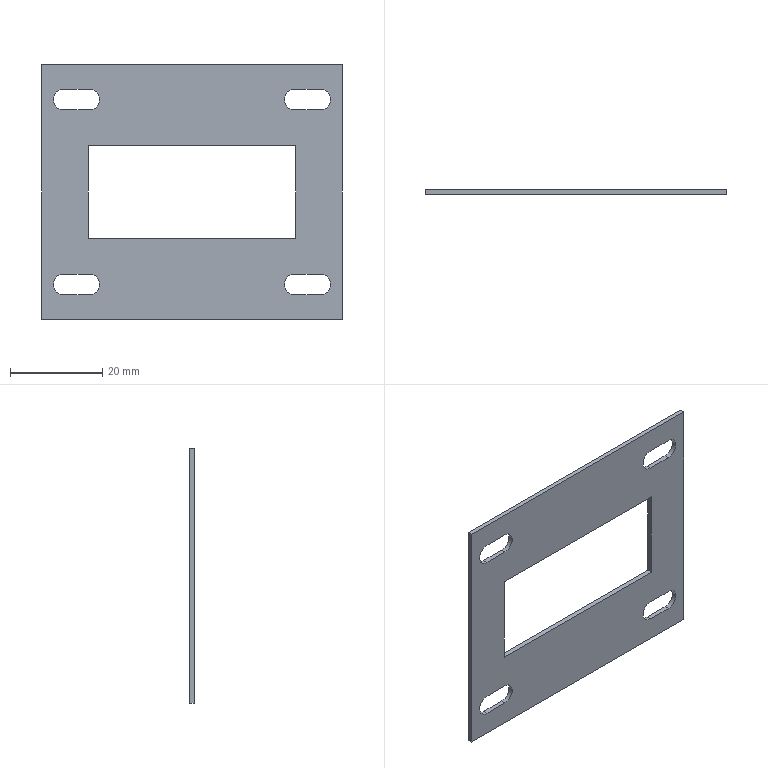Part | STEP file | vibratory feeder support plate | 1 solid | 26 faces | box 65 x 1 x 55 mm | volume 2512 mm3 | plane 18 | cylinder 8 | commonest cylinder face diameters 4.5 x8